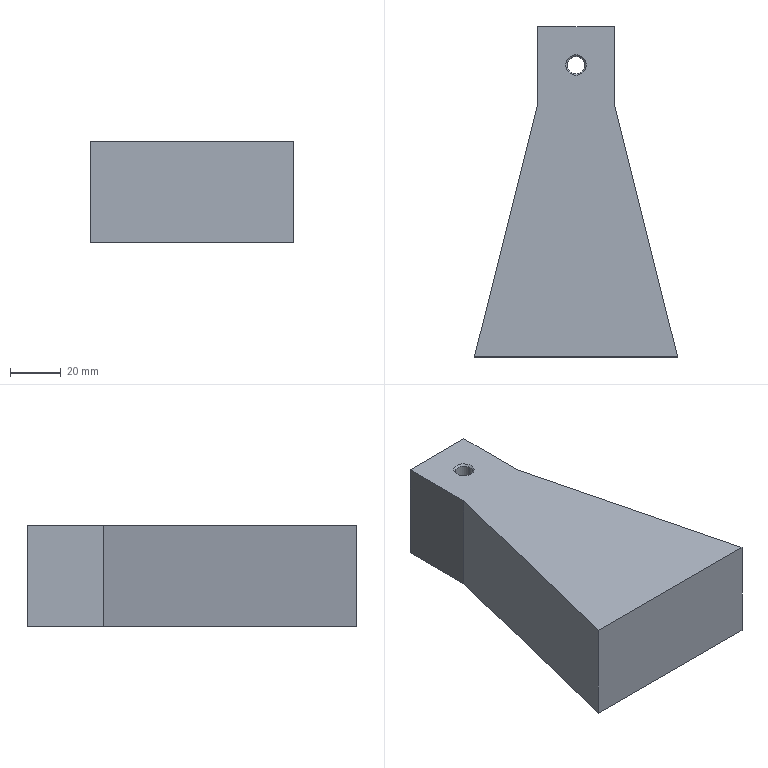Part | SolidWorks | features Extrusion 1, HoleWzd 1 | 1 solid | 12 faces | box 80 x 130 x 40 mm | volume 254543 mm3 | plane 8 | cone 2 | cylinder 2 | commonest cylinder face diameters 6.8 x2
STEP:
#1=CARTESIAN_POINT('',(-3.4,42.273,39.375));
#2=VERTEX_POINT('',#1);
#3=CARTESIAN_POINT('',(3.4,42.273,39.375));
#4=VERTEX_POINT('',#3);
#5=CARTESIAN_POINT('',(0.,42.273,39.375));
#6=DIRECTION('',(0.,0.,1.));
#7=DIRECTION('',(1.,0.,0.));
#8=AXIS2_PLACEMENT_3D('',#5,#6,#7);
#9=CIRCLE('',#8,3.4);
#10=EDGE_CURVE('',#2,#4,#9,.T.);
#11=ORIENTED_EDGE('',*,*,#10,.F.);
#12=CARTESIAN_POINT('',(-4.025,42.273,40.));
#13=VERTEX_POINT('',#12);
#14=CARTESIAN_POINT('',(-4.025,42.273,40.));
#15=DIRECTION('',(-0.7071,0.,0.7071));
#16=VECTOR('',#15,1000.);
#17=LINE('',#14,#16);
#18=EDGE_CURVE('',#2,#13,#17,.T.);
#19=ORIENTED_EDGE('',*,*,#18,.T.);
#20=CARTESIAN_POINT('',(4.025,42.273,40.));
#21=VERTEX_POINT('',#20);
#22=CARTESIAN_POINT('',(0.,42.273,40.));
#23=DIRECTION('',(0.,0.,1.));
#24=DIRECTION('',(1.,0.,0.));
#25=AXIS2_PLACEMENT_3D('',#22,#23,#24);
#26=CIRCLE('',#25,4.025);
#27=EDGE_CURVE('',#13,#21,#26,.T.);
#28=ORIENTED_EDGE('',*,*,#27,.T.);
#29=CARTESIAN_POINT('',(4.025,42.273,40.));
#30=DIRECTION('',(0.7071,0.,0.7071));
#31=VECTOR('',#30,1000.);
#32=LINE('',#29,#31);
#33=EDGE_CURVE('',#4,#21,#32,.T.);
#34=ORIENTED_EDGE('',*,*,#33,.F.);
#35=EDGE_LOOP('',(#11,#19,#28,#34));
#36=FACE_OUTER_BOUND('',#35,.T.);
#37=CARTESIAN_POINT('',(0.,42.273,40.));
#38=DIRECTION('',(0.,0.,1.));
#39=DIRECTION('',(1.,0.,0.));
#40=AXIS2_PLACEMENT_3D('',#37,#38,#39);
#41=CONICAL_SURFACE('',#40,4.025,0.7854);
#42=ADVANCED_FACE('',(#36),#41,.F.);
#43=CARTESIAN_POINT('',(-3.4,42.273,0.));
#44=VERTEX_POINT('',#43);
#45=CARTESIAN_POINT('',(3.4,42.273,0.));
#46=VERTEX_POINT('',#45);
#47=CARTESIAN_POINT('',(0.,42.273,0.));
#48=DIRECTION('',(0.,0.,1.));
#49=DIRECTION('',(1.,0.,0.));
#50=AXIS2_PLACEMENT_3D('',#47,#48,#49);
#51=CIRCLE('',#50,3.4);
#52=EDGE_CURVE('',#44,#46,#51,.T.);
#53=ORIENTED_EDGE('',*,*,#52,.F.);
#54=CARTESIAN_POINT('',(-3.4,42.273,40.));
#55=DIRECTION('',(0.,0.,1.));
#56=VECTOR('',#55,1000.);
#57=LINE('',#54,#56);
#58=EDGE_CURVE('',#44,#2,#57,.T.);
#59=ORIENTED_EDGE('',*,*,#58,.T.);
#60=ORIENTED_EDGE('',*,*,#10,.T.);
#61=CARTESIAN_POINT('',(3.4,42.273,40.));
#62=DIRECTION('',(0.,0.,1.));
#63=VECTOR('',#62,1000.);
#64=LINE('',#61,#63);
#65=EDGE_CURVE('',#46,#4,#64,.T.);
#66=ORIENTED_EDGE('',*,*,#65,.F.);
#67=EDGE_LOOP('',(#53,#59,#60,#66));
#68=FACE_OUTER_BOUND('',#67,.T.);
#69=CARTESIAN_POINT('',(0.,42.273,40.));
#70=DIRECTION('',(0.,0.,1.));
#71=DIRECTION('',(1.,0.,0.));
#72=AXIS2_PLACEMENT_3D('',#69,#70,#71);
#73=CYLINDRICAL_SURFACE('',#72,3.4);
#74=ADVANCED_FACE('',(#68),#73,.F.);
#75=CARTESIAN_POINT('',(-15.,57.273,0.));
#76=VERTEX_POINT('',#75);
#77=CARTESIAN_POINT('',(-15.,27.273,0.));
#78=VERTEX_POINT('',#77);
#79=CARTESIAN_POINT('',(-15.,27.273,0.));
#80=DIRECTION('',(0.,-1.,0.));
#81=VECTOR('',#80,1000.);
#82=LINE('',#79,#81);
#83=EDGE_CURVE('',#76,#78,#82,.T.);
#84=ORIENTED_EDGE('',*,*,#83,.T.);
#85=CARTESIAN_POINT('',(-15.,27.273,40.));
#86=VERTEX_POINT('',#85);
#87=CARTESIAN_POINT('',(-15.,27.273,40.));
#88=DIRECTION('',(0.,0.,-1.));
#89=VECTOR('',#88,1000.);
#90=LINE('',#87,#89);
#91=EDGE_CURVE('',#86,#78,#90,.T.);
#92=ORIENTED_EDGE('',*,*,#91,.F.);
#93=CARTESIAN_POINT('',(-15.,57.273,40.));
#94=VERTEX_POINT('',#93);
#95=CARTESIAN_POINT('',(-15.,27.273,40.));
#96=DIRECTION('',(0.,-1.,0.));
#97=VECTOR('',#96,1000.);
#98=LINE('',#95,#97);
#99=EDGE_CURVE('',#94,#86,#98,.T.);
#100=ORIENTED_EDGE('',*,*,#99,.F.);
#101=CARTESIAN_POINT('',(-15.,57.273,40.));
#102=DIRECTION('',(0.,0.,-1.));
#103=VECTOR('',#102,1000.);
#104=LINE('',#101,#103);
#105=EDGE_CURVE('',#94,#76,#104,.T.);
#106=ORIENTED_EDGE('',*,*,#105,.T.);
#107=EDGE_LOOP('',(#84,#92,#100,#106));
#108=FACE_OUTER_BOUND('',#107,.T.);
#109=CARTESIAN_POINT('',(-15.,27.273,40.));
#110=DIRECTION('',(1.,0.,0.));
#111=DIRECTION('',(0.,0.,-1.));
#112=AXIS2_PLACEMENT_3D('',#109,#110,#111);
#113=PLANE('',#112);
#114=ADVANCED_FACE('',(#108),#113,.F.);
#115=CARTESIAN_POINT('',(-40.,-72.727,0.));
#116=VERTEX_POINT('',#115);
#117=CARTESIAN_POINT('',(-40.,-72.727,0.));
#118=DIRECTION('',(-0.2425,-0.9701,0.));
#119=VECTOR('',#118,1000.);
#120=LINE('',#117,#119);
#121=EDGE_CURVE('',#78,#116,#120,.T.);
#122=ORIENTED_EDGE('',*,*,#121,.T.);
#123=CARTESIAN_POINT('',(-40.,-72.727,40.));
#124=VERTEX_POINT('',#123);
#125=CARTESIAN_POINT('',(-40.,-72.727,40.));
#126=DIRECTION('',(0.,0.,-1.));
#127=VECTOR('',#126,1000.);
#128=LINE('',#125,#127);
#129=EDGE_CURVE('',#124,#116,#128,.T.);
#130=ORIENTED_EDGE('',*,*,#129,.F.);
#131=CARTESIAN_POINT('',(-40.,-72.727,40.));
#132=DIRECTION('',(-0.2425,-0.9701,0.));
#133=VECTOR('',#132,1000.);
#134=LINE('',#131,#133);
#135=EDGE_CURVE('',#86,#124,#134,.T.);
#136=ORIENTED_EDGE('',*,*,#135,.F.);
#137=ORIENTED_EDGE('',*,*,#91,.T.);
#138=EDGE_LOOP('',(#122,#130,#136,#137));
#139=FACE_OUTER_BOUND('',#138,.T.);
#140=CARTESIAN_POINT('',(-40.,-72.727,40.));
#141=DIRECTION('',(0.9701,-0.2425,0.));
#142=DIRECTION('',(0.2425,0.9701,0.));
#143=AXIS2_PLACEMENT_3D('',#140,#141,#142);
#144=PLANE('',#143);
#145=ADVANCED_FACE('',(#139),#144,.F.);
#146=CARTESIAN_POINT('',(40.,-72.727,0.));
#147=VERTEX_POINT('',#146);
#148=CARTESIAN_POINT('',(40.,-72.727,0.));
#149=DIRECTION('',(1.,0.,0.));
#150=VECTOR('',#149,1000.);
#151=LINE('',#148,#150);
#152=EDGE_CURVE('',#116,#147,#151,.T.);
#153=ORIENTED_EDGE('',*,*,#152,.T.);
#154=CARTESIAN_POINT('',(40.,-72.727,40.));
#155=VERTEX_POINT('',#154);
#156=CARTESIAN_POINT('',(40.,-72.727,40.));
#157=DIRECTION('',(0.,0.,-1.));
#158=VECTOR('',#157,1000.);
#159=LINE('',#156,#158);
#160=EDGE_CURVE('',#155,#147,#159,.T.);
#161=ORIENTED_EDGE('',*,*,#160,.F.);
#162=CARTESIAN_POINT('',(40.,-72.727,40.));
#163=DIRECTION('',(1.,0.,0.));
#164=VECTOR('',#163,1000.);
#165=LINE('',#162,#164);
#166=EDGE_CURVE('',#124,#155,#165,.T.);
#167=ORIENTED_EDGE('',*,*,#166,.F.);
#168=ORIENTED_EDGE('',*,*,#129,.T.);
#169=EDGE_LOOP('',(#153,#161,#167,#168));
#170=FACE_OUTER_BOUND('',#169,.T.);
#171=CARTESIAN_POINT('',(40.,-72.727,40.));
#172=DIRECTION('',(0.,1.,0.));
#173=DIRECTION('',(-1.,0.,0.));
#174=AXIS2_PLACEMENT_3D('',#171,#172,#173);
#175=PLANE('',#174);
#176=ADVANCED_FACE('',(#170),#175,.F.);
#177=CARTESIAN_POINT('',(15.,27.273,0.));
#178=VERTEX_POINT('',#177);
#179=CARTESIAN_POINT('',(40.,-72.727,0.));
#180=DIRECTION('',(-0.2425,0.9701,0.));
#181=VECTOR('',#180,1000.);
#182=LINE('',#179,#181);
#183=EDGE_CURVE('',#147,#178,#182,.T.);
#184=ORIENTED_EDGE('',*,*,#183,.T.);
#185=CARTESIAN_POINT('',(15.,27.273,40.));
#186=VERTEX_POINT('',#185);
#187=CARTESIAN_POINT('',(15.,27.273,40.));
#188=DIRECTION('',(0.,0.,-1.));
#189=VECTOR('',#188,1000.);
#190=LINE('',#187,#189);
#191=EDGE_CURVE('',#186,#178,#190,.T.);
#192=ORIENTED_EDGE('',*,*,#191,.F.);
#193=CARTESIAN_POINT('',(40.,-72.727,40.));
#194=DIRECTION('',(-0.2425,0.9701,0.));
#195=VECTOR('',#194,1000.);
#196=LINE('',#193,#195);
#197=EDGE_CURVE('',#155,#186,#196,.T.);
#198=ORIENTED_EDGE('',*,*,#197,.F.);
#199=ORIENTED_EDGE('',*,*,#160,.T.);
#200=EDGE_LOOP('',(#184,#192,#198,#199));
#201=FACE_OUTER_BOUND('',#200,.T.);
#202=CARTESIAN_POINT('',(40.,-72.727,40.));
#203=DIRECTION('',(-0.9701,-0.2425,0.));
#204=DIRECTION('',(0.2425,-0.9701,0.));
#205=AXIS2_PLACEMENT_3D('',#202,#203,#204);
#206=PLANE('',#205);
#207=ADVANCED_FACE('',(#201),#206,.F.);
#208=CARTESIAN_POINT('',(15.,57.273,0.));
#209=VERTEX_POINT('',#208);
#210=CARTESIAN_POINT('',(15.,57.273,0.));
#211=DIRECTION('',(0.,1.,0.));
#212=VECTOR('',#211,1000.);
#213=LINE('',#210,#212);
#214=EDGE_CURVE('',#178,#209,#213,.T.);
#215=ORIENTED_EDGE('',*,*,#214,.T.);
#216=CARTESIAN_POINT('',(15.,57.273,40.));
#217=VERTEX_POINT('',#216);
#218=CARTESIAN_POINT('',(15.,57.273,40.));
#219=DIRECTION('',(0.,0.,-1.));
#220=VECTOR('',#219,1000.);
#221=LINE('',#218,#220);
#222=EDGE_CURVE('',#217,#209,#221,.T.);
#223=ORIENTED_EDGE('',*,*,#222,.F.);
#224=CARTESIAN_POINT('',(15.,57.273,40.));
#225=DIRECTION('',(0.,1.,0.));
#226=VECTOR('',#225,1000.);
#227=LINE('',#224,#226);
#228=EDGE_CURVE('',#186,#217,#227,.T.);
#229=ORIENTED_EDGE('',*,*,#228,.F.);
#230=ORIENTED_EDGE('',*,*,#191,.T.);
#231=EDGE_LOOP('',(#215,#223,#229,#230));
#232=FACE_OUTER_BOUND('',#231,.T.);
#233=CARTESIAN_POINT('',(15.,57.273,40.));
#234=DIRECTION('',(-1.,0.,0.));
#235=DIRECTION('',(0.,-1.,0.));
#236=AXIS2_PLACEMENT_3D('',#233,#234,#235);
#237=PLANE('',#236);
#238=ADVANCED_FACE('',(#232),#237,.F.);
#239=CARTESIAN_POINT('',(-15.,57.273,0.));
#240=DIRECTION('',(-1.,0.,0.));
#241=VECTOR('',#240,1000.);
#242=LINE('',#239,#241);
#243=EDGE_CURVE('',#209,#76,#242,.T.);
#244=ORIENTED_EDGE('',*,*,#243,.T.);
#245=ORIENTED_EDGE('',*,*,#105,.F.);
#246=CARTESIAN_POINT('',(-15.,57.273,40.));
#247=DIRECTION('',(-1.,0.,0.));
#248=VECTOR('',#247,1000.);
#249=LINE('',#246,#248);
#250=EDGE_CURVE('',#217,#94,#249,.T.);
#251=ORIENTED_EDGE('',*,*,#250,.F.);
#252=ORIENTED_EDGE('',*,*,#222,.T.);
#253=EDGE_LOOP('',(#244,#245,#251,#252));
#254=FACE_OUTER_BOUND('',#253,.T.);
#255=CARTESIAN_POINT('',(-15.,57.273,40.));
#256=DIRECTION('',(0.,-1.,0.));
#257=DIRECTION('',(1.,0.,0.));
#258=AXIS2_PLACEMENT_3D('',#255,#256,#257);
#259=PLANE('',#258);
#260=ADVANCED_FACE('',(#254),#259,.F.);
#261=CARTESIAN_POINT('',(0.,42.273,40.));
#262=DIRECTION('',(0.,0.,1.));
#263=DIRECTION('',(1.,0.,0.));
#264=AXIS2_PLACEMENT_3D('',#261,#262,#263);
#265=CIRCLE('',#264,4.025);
#266=EDGE_CURVE('',#21,#13,#265,.T.);
#267=ORIENTED_EDGE('',*,*,#266,.F.);
#268=ORIENTED_EDGE('',*,*,#27,.F.);
#269=EDGE_LOOP('',(#267,#268));
#270=FACE_BOUND('',#269,.T.);
#271=ORIENTED_EDGE('',*,*,#99,.T.);
#272=ORIENTED_EDGE('',*,*,#135,.T.);
#273=ORIENTED_EDGE('',*,*,#166,.T.);
#274=ORIENTED_EDGE('',*,*,#197,.T.);
#275=ORIENTED_EDGE('',*,*,#228,.T.);
#276=ORIENTED_EDGE('',*,*,#250,.T.);
#277=EDGE_LOOP('',(#271,#272,#273,#274,#275,#276));
#278=FACE_OUTER_BOUND('',#277,.T.);
#279=CARTESIAN_POINT('',(0.,0.,40.));
#280=DIRECTION('',(0.,0.,-1.));
#281=DIRECTION('',(-1.,0.,0.));
#282=AXIS2_PLACEMENT_3D('',#279,#280,#281);
#283=PLANE('',#282);
#284=ADVANCED_FACE('',(#270,#278),#283,.F.);
#285=CARTESIAN_POINT('',(0.,42.273,0.));
#286=DIRECTION('',(0.,0.,1.));
#287=DIRECTION('',(1.,0.,0.));
#288=AXIS2_PLACEMENT_3D('',#285,#286,#287);
#289=CIRCLE('',#288,3.4);
#290=EDGE_CURVE('',#46,#44,#289,.T.);
#291=ORIENTED_EDGE('',*,*,#290,.T.);
#292=ORIENTED_EDGE('',*,*,#52,.T.);
#293=EDGE_LOOP('',(#291,#292));
#294=FACE_BOUND('',#293,.T.);
#295=ORIENTED_EDGE('',*,*,#83,.F.);
#296=ORIENTED_EDGE('',*,*,#243,.F.);
#297=ORIENTED_EDGE('',*,*,#214,.F.);
#298=ORIENTED_EDGE('',*,*,#183,.F.);
#299=ORIENTED_EDGE('',*,*,#152,.F.);
#300=ORIENTED_EDGE('',*,*,#121,.F.);
#301=EDGE_LOOP('',(#295,#296,#297,#298,#299,#300));
#302=FACE_OUTER_BOUND('',#301,.T.);
#303=CARTESIAN_POINT('',(0.,0.,0.));
#304=DIRECTION('',(0.,0.,-1.));
#305=DIRECTION('',(-1.,0.,0.));
#306=AXIS2_PLACEMENT_3D('',#303,#304,#305);
#307=PLANE('',#306);
#308=ADVANCED_FACE('',(#294,#302),#307,.T.);
#309=ORIENTED_EDGE('',*,*,#58,.F.);
#310=ORIENTED_EDGE('',*,*,#290,.F.);
#311=ORIENTED_EDGE('',*,*,#65,.T.);
#312=CARTESIAN_POINT('',(0.,42.273,39.375));
#313=DIRECTION('',(0.,0.,1.));
#314=DIRECTION('',(1.,0.,0.));
#315=AXIS2_PLACEMENT_3D('',#312,#313,#314);
#316=CIRCLE('',#315,3.4);
#317=EDGE_CURVE('',#4,#2,#316,.T.);
#318=ORIENTED_EDGE('',*,*,#317,.T.);
#319=EDGE_LOOP('',(#309,#310,#311,#318));
#320=FACE_OUTER_BOUND('',#319,.T.);
#321=CARTESIAN_POINT('',(0.,42.273,40.));
#322=DIRECTION('',(0.,0.,1.));
#323=DIRECTION('',(1.,0.,0.));
#324=AXIS2_PLACEMENT_3D('',#321,#322,#323);
#325=CYLINDRICAL_SURFACE('',#324,3.4);
#326=ADVANCED_FACE('',(#320),#325,.F.);
#327=ORIENTED_EDGE('',*,*,#18,.F.);
#328=ORIENTED_EDGE('',*,*,#317,.F.);
#329=ORIENTED_EDGE('',*,*,#33,.T.);
#330=ORIENTED_EDGE('',*,*,#266,.T.);
#331=EDGE_LOOP('',(#327,#328,#329,#330));
#332=FACE_OUTER_BOUND('',#331,.T.);
#333=CARTESIAN_POINT('',(0.,42.273,40.));
#334=DIRECTION('',(0.,0.,1.));
#335=DIRECTION('',(1.,0.,0.));
#336=AXIS2_PLACEMENT_3D('',#333,#334,#335);
#337=CONICAL_SURFACE('',#336,4.025,0.7854);
#338=ADVANCED_FACE('',(#332),#337,.F.);
#339=CLOSED_SHELL('',(#42,#74,#114,#145,#176,#207,#238,#260,#284,#308,#326,#338));
#340=MANIFOLD_SOLID_BREP('',#339);
#341=CARTESIAN_POINT('',(0.,0.,0.));
#342=DIRECTION('',(0.,0.,1.));
#343=DIRECTION('',(1.,0.,0.));
#344=AXIS2_PLACEMENT_3D('',#341,#342,#343);
#345=(LENGTH_UNIT()NAMED_UNIT(*)SI_UNIT(.MILLI.,.METRE.));
#346=UNCERTAINTY_MEASURE_WITH_UNIT(LENGTH_MEASURE(0.00001),#345,'','');
#347=(NAMED_UNIT(*)PLANE_ANGLE_UNIT()SI_UNIT($,.RADIAN.));
#348=(NAMED_UNIT(*)SI_UNIT($,.STERADIAN.)SOLID_ANGLE_UNIT());
#349=(GEOMETRIC_REPRESENTATION_CONTEXT(3)GLOBAL_UNCERTAINTY_ASSIGNED_CONTEXT((#346))GLOBAL_UNIT_ASSIGNED_CONTEXT((#345,#347,#348))REPRESENTATION_CONTEXT('',''));
#350=ADVANCED_BREP_SHAPE_REPRESENTATION('',(#340,#344),#349);